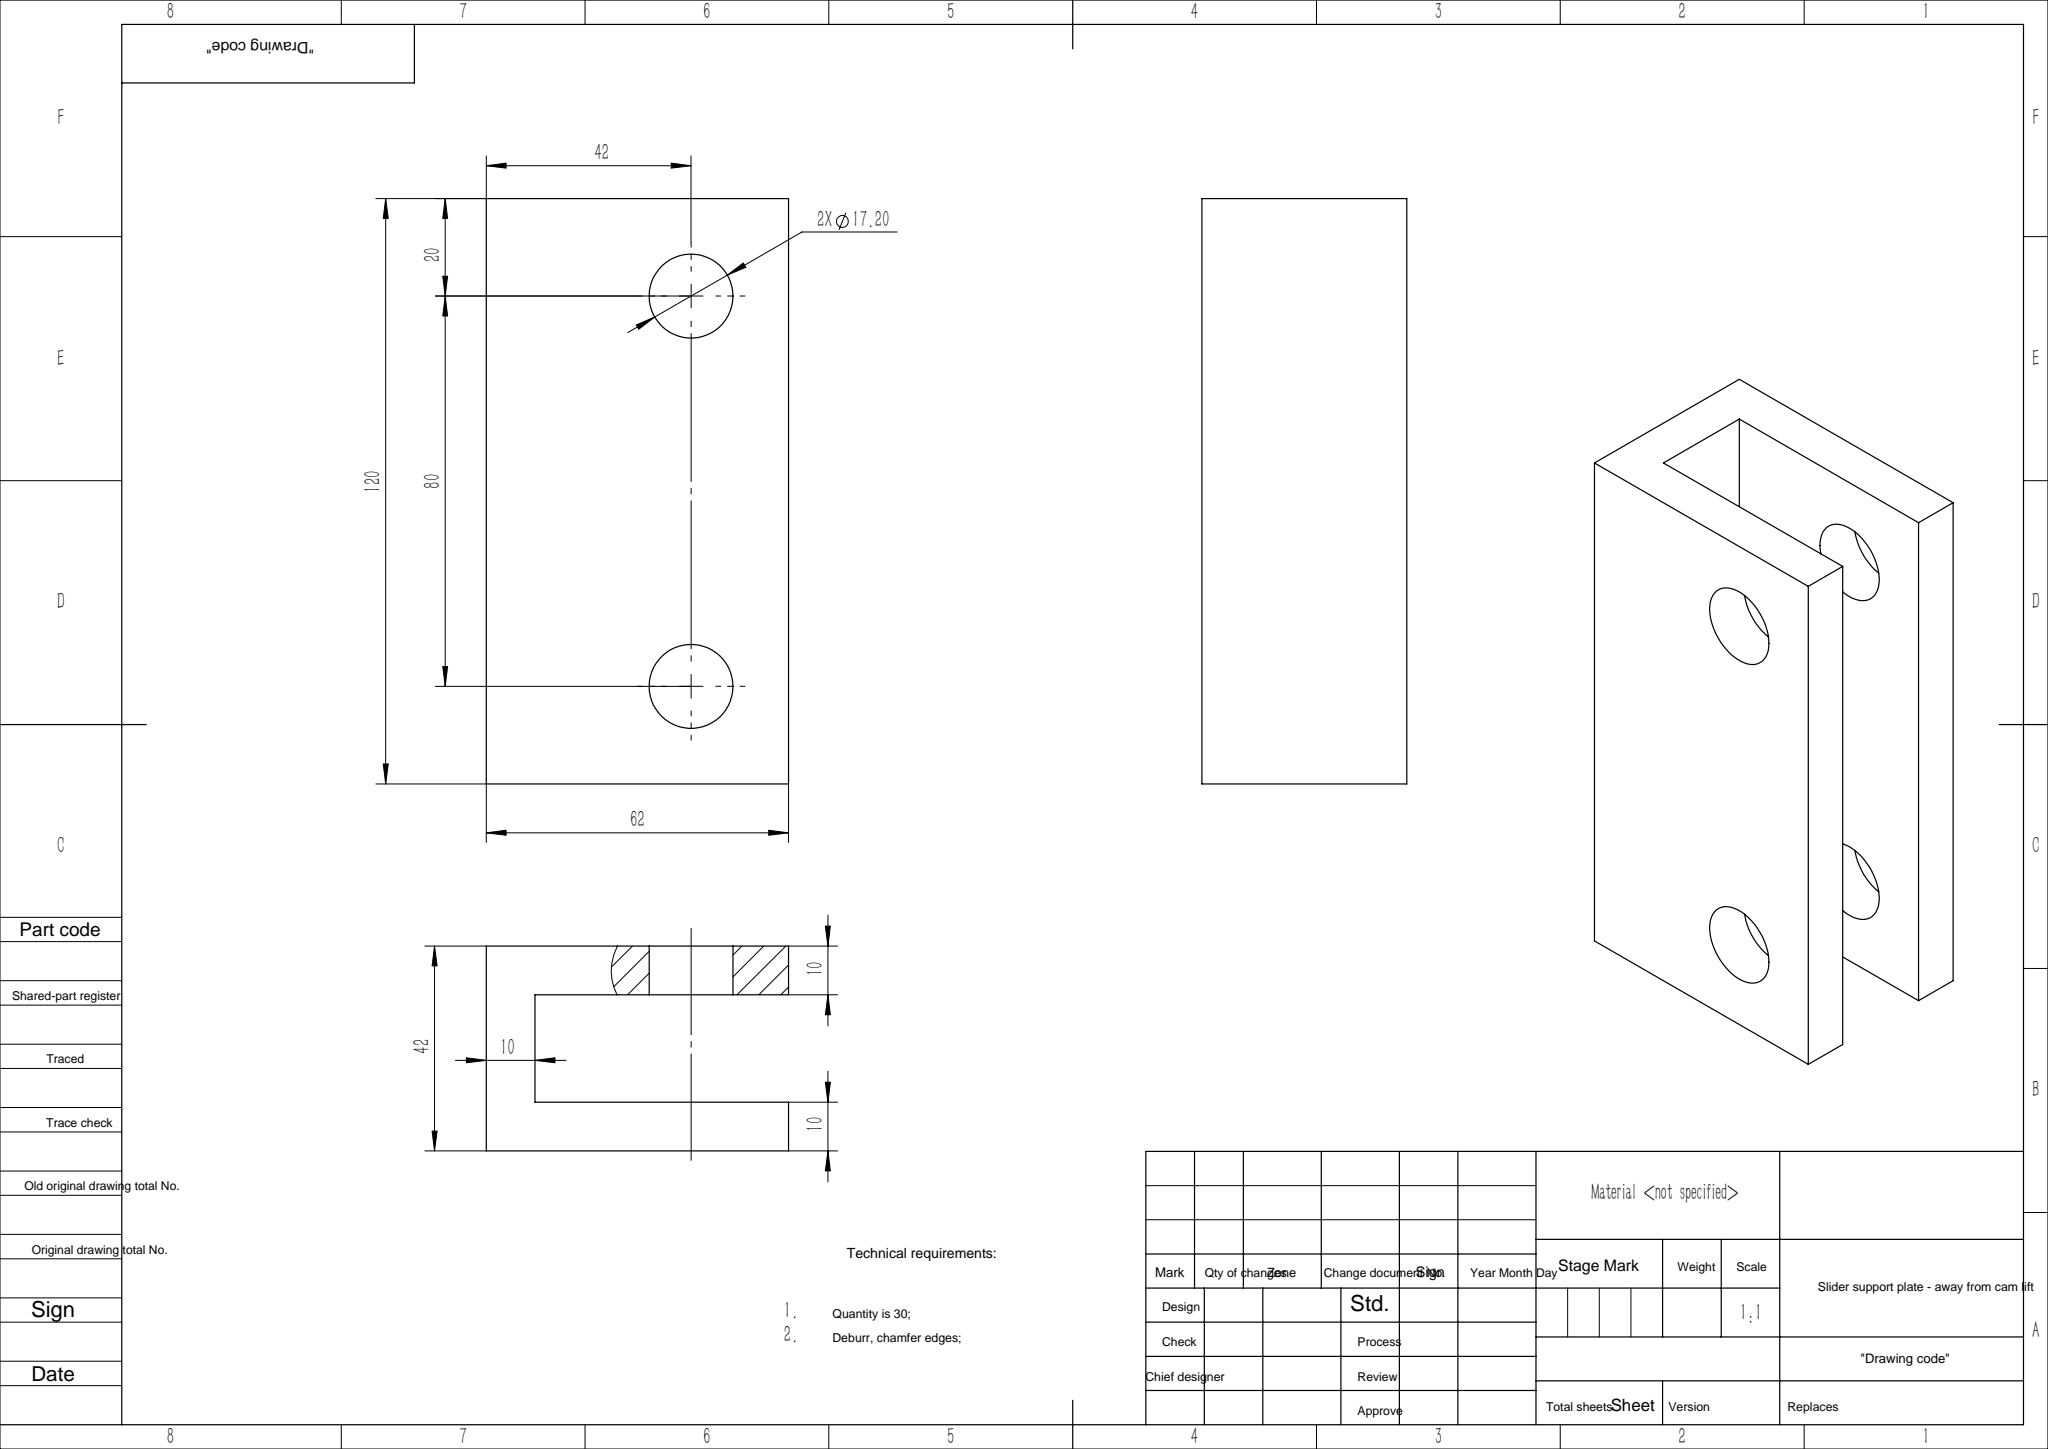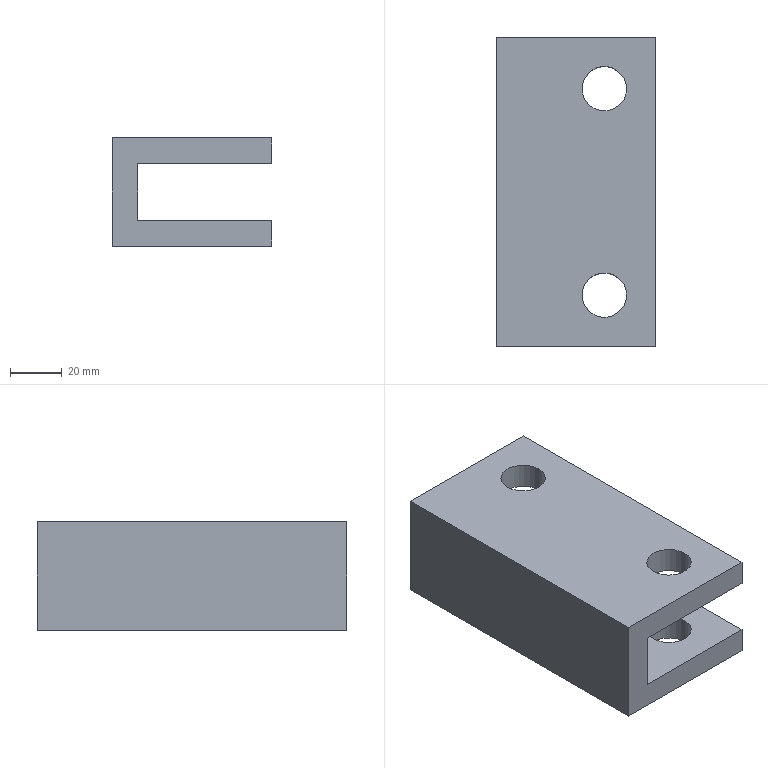Part | SolidWorks | features Extrusion 1, ICE 1 | 1 solid | 18 faces | box 62 x 120 x 42 mm | volume 165906 mm3 | plane 10 | cylinder 8 | commonest cylinder face diameters 17.2 x8
STEP:
#1=CARTESIAN_POINT('',(33.4,20.,11.));
#2=VERTEX_POINT('',#1);
#3=CARTESIAN_POINT('',(50.6,20.,11.));
#4=VERTEX_POINT('',#3);
#5=CARTESIAN_POINT('',(42.,20.,11.));
#6=DIRECTION('',(0.,0.,1.));
#7=DIRECTION('',(1.,0.,0.));
#8=AXIS2_PLACEMENT_3D('',#5,#6,#7);
#9=CIRCLE('',#8,8.6);
#10=EDGE_CURVE('',#2,#4,#9,.T.);
#11=ORIENTED_EDGE('',*,*,#10,.F.);
#12=CARTESIAN_POINT('',(33.4,20.,21.));
#13=VERTEX_POINT('',#12);
#14=CARTESIAN_POINT('',(33.4,20.,-21.));
#15=DIRECTION('',(0.,0.,1.));
#16=VECTOR('',#15,1000.);
#17=LINE('',#14,#16);
#18=EDGE_CURVE('',#2,#13,#17,.T.);
#19=ORIENTED_EDGE('',*,*,#18,.T.);
#20=CARTESIAN_POINT('',(50.6,20.,21.));
#21=VERTEX_POINT('',#20);
#22=CARTESIAN_POINT('',(42.,20.,21.));
#23=DIRECTION('',(0.,0.,1.));
#24=DIRECTION('',(1.,0.,0.));
#25=AXIS2_PLACEMENT_3D('',#22,#23,#24);
#26=CIRCLE('',#25,8.6);
#27=EDGE_CURVE('',#13,#21,#26,.T.);
#28=ORIENTED_EDGE('',*,*,#27,.T.);
#29=CARTESIAN_POINT('',(50.6,20.,-21.));
#30=DIRECTION('',(0.,0.,1.));
#31=VECTOR('',#30,1000.);
#32=LINE('',#29,#31);
#33=EDGE_CURVE('',#4,#21,#32,.T.);
#34=ORIENTED_EDGE('',*,*,#33,.F.);
#35=EDGE_LOOP('',(#11,#19,#28,#34));
#36=FACE_OUTER_BOUND('',#35,.T.);
#37=CARTESIAN_POINT('',(42.,20.,-21.));
#38=DIRECTION('',(0.,0.,1.));
#39=DIRECTION('',(1.,0.,0.));
#40=AXIS2_PLACEMENT_3D('',#37,#38,#39);
#41=CYLINDRICAL_SURFACE('',#40,8.6);
#42=ADVANCED_FACE('',(#36),#41,.F.);
#43=CARTESIAN_POINT('',(33.4,20.,-21.));
#44=VERTEX_POINT('',#43);
#45=CARTESIAN_POINT('',(50.6,20.,-21.));
#46=VERTEX_POINT('',#45);
#47=CARTESIAN_POINT('',(42.,20.,-21.));
#48=DIRECTION('',(0.,0.,1.));
#49=DIRECTION('',(1.,0.,0.));
#50=AXIS2_PLACEMENT_3D('',#47,#48,#49);
#51=CIRCLE('',#50,8.6);
#52=EDGE_CURVE('',#44,#46,#51,.T.);
#53=ORIENTED_EDGE('',*,*,#52,.F.);
#54=CARTESIAN_POINT('',(33.4,20.,-11.));
#55=VERTEX_POINT('',#54);
#56=CARTESIAN_POINT('',(33.4,20.,-21.));
#57=DIRECTION('',(0.,0.,1.));
#58=VECTOR('',#57,1000.);
#59=LINE('',#56,#58);
#60=EDGE_CURVE('',#44,#55,#59,.T.);
#61=ORIENTED_EDGE('',*,*,#60,.T.);
#62=CARTESIAN_POINT('',(50.6,20.,-11.));
#63=VERTEX_POINT('',#62);
#64=CARTESIAN_POINT('',(42.,20.,-11.));
#65=DIRECTION('',(0.,0.,-1.));
#66=DIRECTION('',(-1.,0.,0.));
#67=AXIS2_PLACEMENT_3D('',#64,#65,#66);
#68=CIRCLE('',#67,8.6);
#69=EDGE_CURVE('',#63,#55,#68,.T.);
#70=ORIENTED_EDGE('',*,*,#69,.F.);
#71=CARTESIAN_POINT('',(50.6,20.,-21.));
#72=DIRECTION('',(0.,0.,1.));
#73=VECTOR('',#72,1000.);
#74=LINE('',#71,#73);
#75=EDGE_CURVE('',#46,#63,#74,.T.);
#76=ORIENTED_EDGE('',*,*,#75,.F.);
#77=EDGE_LOOP('',(#53,#61,#70,#76));
#78=FACE_OUTER_BOUND('',#77,.T.);
#79=CARTESIAN_POINT('',(42.,20.,-21.));
#80=DIRECTION('',(0.,0.,1.));
#81=DIRECTION('',(1.,0.,0.));
#82=AXIS2_PLACEMENT_3D('',#79,#80,#81);
#83=CYLINDRICAL_SURFACE('',#82,8.6);
#84=ADVANCED_FACE('',(#78),#83,.F.);
#85=CARTESIAN_POINT('',(33.4,100.,11.));
#86=VERTEX_POINT('',#85);
#87=CARTESIAN_POINT('',(50.6,100.,11.));
#88=VERTEX_POINT('',#87);
#89=CARTESIAN_POINT('',(42.,100.,11.));
#90=DIRECTION('',(0.,0.,1.));
#91=DIRECTION('',(1.,0.,0.));
#92=AXIS2_PLACEMENT_3D('',#89,#90,#91);
#93=CIRCLE('',#92,8.6);
#94=EDGE_CURVE('',#86,#88,#93,.T.);
#95=ORIENTED_EDGE('',*,*,#94,.F.);
#96=CARTESIAN_POINT('',(33.4,100.,21.));
#97=VERTEX_POINT('',#96);
#98=CARTESIAN_POINT('',(33.4,100.,-21.));
#99=DIRECTION('',(0.,0.,1.));
#100=VECTOR('',#99,1000.);
#101=LINE('',#98,#100);
#102=EDGE_CURVE('',#86,#97,#101,.T.);
#103=ORIENTED_EDGE('',*,*,#102,.T.);
#104=CARTESIAN_POINT('',(50.6,100.,21.));
#105=VERTEX_POINT('',#104);
#106=CARTESIAN_POINT('',(42.,100.,21.));
#107=DIRECTION('',(0.,0.,1.));
#108=DIRECTION('',(1.,0.,0.));
#109=AXIS2_PLACEMENT_3D('',#106,#107,#108);
#110=CIRCLE('',#109,8.6);
#111=EDGE_CURVE('',#97,#105,#110,.T.);
#112=ORIENTED_EDGE('',*,*,#111,.T.);
#113=CARTESIAN_POINT('',(50.6,100.,-21.));
#114=DIRECTION('',(0.,0.,1.));
#115=VECTOR('',#114,1000.);
#116=LINE('',#113,#115);
#117=EDGE_CURVE('',#88,#105,#116,.T.);
#118=ORIENTED_EDGE('',*,*,#117,.F.);
#119=EDGE_LOOP('',(#95,#103,#112,#118));
#120=FACE_OUTER_BOUND('',#119,.T.);
#121=CARTESIAN_POINT('',(42.,100.,-21.));
#122=DIRECTION('',(0.,0.,1.));
#123=DIRECTION('',(1.,0.,0.));
#124=AXIS2_PLACEMENT_3D('',#121,#122,#123);
#125=CYLINDRICAL_SURFACE('',#124,8.6);
#126=ADVANCED_FACE('',(#120),#125,.F.);
#127=CARTESIAN_POINT('',(33.4,100.,-21.));
#128=VERTEX_POINT('',#127);
#129=CARTESIAN_POINT('',(50.6,100.,-21.));
#130=VERTEX_POINT('',#129);
#131=CARTESIAN_POINT('',(42.,100.,-21.));
#132=DIRECTION('',(0.,0.,1.));
#133=DIRECTION('',(1.,0.,0.));
#134=AXIS2_PLACEMENT_3D('',#131,#132,#133);
#135=CIRCLE('',#134,8.6);
#136=EDGE_CURVE('',#128,#130,#135,.T.);
#137=ORIENTED_EDGE('',*,*,#136,.F.);
#138=CARTESIAN_POINT('',(33.4,100.,-11.));
#139=VERTEX_POINT('',#138);
#140=CARTESIAN_POINT('',(33.4,100.,-21.));
#141=DIRECTION('',(0.,0.,1.));
#142=VECTOR('',#141,1000.);
#143=LINE('',#140,#142);
#144=EDGE_CURVE('',#128,#139,#143,.T.);
#145=ORIENTED_EDGE('',*,*,#144,.T.);
#146=CARTESIAN_POINT('',(50.6,100.,-11.));
#147=VERTEX_POINT('',#146);
#148=CARTESIAN_POINT('',(42.,100.,-11.));
#149=DIRECTION('',(0.,0.,-1.));
#150=DIRECTION('',(-1.,0.,0.));
#151=AXIS2_PLACEMENT_3D('',#148,#149,#150);
#152=CIRCLE('',#151,8.6);
#153=EDGE_CURVE('',#147,#139,#152,.T.);
#154=ORIENTED_EDGE('',*,*,#153,.F.);
#155=CARTESIAN_POINT('',(50.6,100.,-21.));
#156=DIRECTION('',(0.,0.,1.));
#157=VECTOR('',#156,1000.);
#158=LINE('',#155,#157);
#159=EDGE_CURVE('',#130,#147,#158,.T.);
#160=ORIENTED_EDGE('',*,*,#159,.F.);
#161=EDGE_LOOP('',(#137,#145,#154,#160));
#162=FACE_OUTER_BOUND('',#161,.T.);
#163=CARTESIAN_POINT('',(42.,100.,-21.));
#164=DIRECTION('',(0.,0.,1.));
#165=DIRECTION('',(1.,0.,0.));
#166=AXIS2_PLACEMENT_3D('',#163,#164,#165);
#167=CYLINDRICAL_SURFACE('',#166,8.6);
#168=ADVANCED_FACE('',(#162),#167,.F.);
#169=CARTESIAN_POINT('',(0.,0.,-21.));
#170=VERTEX_POINT('',#169);
#171=CARTESIAN_POINT('',(0.,0.,21.));
#172=VERTEX_POINT('',#171);
#173=CARTESIAN_POINT('',(0.,0.,-21.));
#174=DIRECTION('',(0.,0.,1.));
#175=VECTOR('',#174,1000.);
#176=LINE('',#173,#175);
#177=EDGE_CURVE('',#170,#172,#176,.T.);
#178=ORIENTED_EDGE('',*,*,#177,.T.);
#179=CARTESIAN_POINT('',(0.,120.,21.));
#180=VERTEX_POINT('',#179);
#181=CARTESIAN_POINT('',(0.,120.,21.));
#182=DIRECTION('',(0.,-1.,0.));
#183=VECTOR('',#182,1000.);
#184=LINE('',#181,#183);
#185=EDGE_CURVE('',#180,#172,#184,.T.);
#186=ORIENTED_EDGE('',*,*,#185,.F.);
#187=CARTESIAN_POINT('',(0.,120.,-21.));
#188=VERTEX_POINT('',#187);
#189=CARTESIAN_POINT('',(0.,120.,-21.));
#190=DIRECTION('',(0.,0.,1.));
#191=VECTOR('',#190,1000.);
#192=LINE('',#189,#191);
#193=EDGE_CURVE('',#188,#180,#192,.T.);
#194=ORIENTED_EDGE('',*,*,#193,.F.);
#195=CARTESIAN_POINT('',(0.,120.,-21.));
#196=DIRECTION('',(0.,-1.,0.));
#197=VECTOR('',#196,1000.);
#198=LINE('',#195,#197);
#199=EDGE_CURVE('',#188,#170,#198,.T.);
#200=ORIENTED_EDGE('',*,*,#199,.T.);
#201=EDGE_LOOP('',(#178,#186,#194,#200));
#202=FACE_OUTER_BOUND('',#201,.T.);
#203=CARTESIAN_POINT('',(0.,120.,-21.));
#204=DIRECTION('',(1.,0.,0.));
#205=DIRECTION('',(0.,0.,-1.));
#206=AXIS2_PLACEMENT_3D('',#203,#204,#205);
#207=PLANE('',#206);
#208=ADVANCED_FACE('',(#202),#207,.F.);
#209=CARTESIAN_POINT('',(42.,20.,21.));
#210=DIRECTION('',(0.,0.,1.));
#211=DIRECTION('',(1.,0.,0.));
#212=AXIS2_PLACEMENT_3D('',#209,#210,#211);
#213=CIRCLE('',#212,8.6);
#214=EDGE_CURVE('',#21,#13,#213,.T.);
#215=ORIENTED_EDGE('',*,*,#214,.F.);
#216=ORIENTED_EDGE('',*,*,#27,.F.);
#217=EDGE_LOOP('',(#215,#216));
#218=FACE_BOUND('',#217,.T.);
#219=CARTESIAN_POINT('',(42.,100.,21.));
#220=DIRECTION('',(0.,0.,1.));
#221=DIRECTION('',(1.,0.,0.));
#222=AXIS2_PLACEMENT_3D('',#219,#220,#221);
#223=CIRCLE('',#222,8.6);
#224=EDGE_CURVE('',#105,#97,#223,.T.);
#225=ORIENTED_EDGE('',*,*,#224,.F.);
#226=ORIENTED_EDGE('',*,*,#111,.F.);
#227=EDGE_LOOP('',(#225,#226));
#228=FACE_BOUND('',#227,.T.);
#229=CARTESIAN_POINT('',(62.,0.,21.));
#230=VERTEX_POINT('',#229);
#231=CARTESIAN_POINT('',(0.,0.,21.));
#232=DIRECTION('',(1.,0.,0.));
#233=VECTOR('',#232,1000.);
#234=LINE('',#231,#233);
#235=EDGE_CURVE('',#172,#230,#234,.T.);
#236=ORIENTED_EDGE('',*,*,#235,.T.);
#237=CARTESIAN_POINT('',(62.,120.,21.));
#238=VERTEX_POINT('',#237);
#239=CARTESIAN_POINT('',(62.,120.,21.));
#240=DIRECTION('',(0.,-1.,0.));
#241=VECTOR('',#240,1000.);
#242=LINE('',#239,#241);
#243=EDGE_CURVE('',#238,#230,#242,.T.);
#244=ORIENTED_EDGE('',*,*,#243,.F.);
#245=CARTESIAN_POINT('',(0.,120.,21.));
#246=DIRECTION('',(1.,0.,0.));
#247=VECTOR('',#246,1000.);
#248=LINE('',#245,#247);
#249=EDGE_CURVE('',#180,#238,#248,.T.);
#250=ORIENTED_EDGE('',*,*,#249,.F.);
#251=ORIENTED_EDGE('',*,*,#185,.T.);
#252=EDGE_LOOP('',(#236,#244,#250,#251));
#253=FACE_OUTER_BOUND('',#252,.T.);
#254=CARTESIAN_POINT('',(0.,120.,21.));
#255=DIRECTION('',(0.,0.,-1.));
#256=DIRECTION('',(-1.,0.,0.));
#257=AXIS2_PLACEMENT_3D('',#254,#255,#256);
#258=PLANE('',#257);
#259=ADVANCED_FACE('',(#218,#228,#253),#258,.F.);
#260=CARTESIAN_POINT('',(62.,0.,11.));
#261=VERTEX_POINT('',#260);
#262=CARTESIAN_POINT('',(62.,0.,11.));
#263=DIRECTION('',(0.,0.,-1.));
#264=VECTOR('',#263,1000.);
#265=LINE('',#262,#264);
#266=EDGE_CURVE('',#230,#261,#265,.T.);
#267=ORIENTED_EDGE('',*,*,#266,.T.);
#268=CARTESIAN_POINT('',(62.,120.,11.));
#269=VERTEX_POINT('',#268);
#270=CARTESIAN_POINT('',(62.,120.,11.));
#271=DIRECTION('',(0.,-1.,0.));
#272=VECTOR('',#271,1000.);
#273=LINE('',#270,#272);
#274=EDGE_CURVE('',#269,#261,#273,.T.);
#275=ORIENTED_EDGE('',*,*,#274,.F.);
#276=CARTESIAN_POINT('',(62.,120.,11.));
#277=DIRECTION('',(0.,0.,-1.));
#278=VECTOR('',#277,1000.);
#279=LINE('',#276,#278);
#280=EDGE_CURVE('',#238,#269,#279,.T.);
#281=ORIENTED_EDGE('',*,*,#280,.F.);
#282=ORIENTED_EDGE('',*,*,#243,.T.);
#283=EDGE_LOOP('',(#267,#275,#281,#282));
#284=FACE_OUTER_BOUND('',#283,.T.);
#285=CARTESIAN_POINT('',(62.,120.,11.));
#286=DIRECTION('',(-1.,0.,0.));
#287=DIRECTION('',(0.,0.,1.));
#288=AXIS2_PLACEMENT_3D('',#285,#286,#287);
#289=PLANE('',#288);
#290=ADVANCED_FACE('',(#284),#289,.F.);
#291=CARTESIAN_POINT('',(42.,20.,11.));
#292=DIRECTION('',(0.,0.,1.));
#293=DIRECTION('',(1.,0.,0.));
#294=AXIS2_PLACEMENT_3D('',#291,#292,#293);
#295=CIRCLE('',#294,8.6);
#296=EDGE_CURVE('',#4,#2,#295,.T.);
#297=ORIENTED_EDGE('',*,*,#296,.T.);
#298=ORIENTED_EDGE('',*,*,#10,.T.);
#299=EDGE_LOOP('',(#297,#298));
#300=FACE_BOUND('',#299,.T.);
#301=CARTESIAN_POINT('',(42.,100.,11.));
#302=DIRECTION('',(0.,0.,1.));
#303=DIRECTION('',(1.,0.,0.));
#304=AXIS2_PLACEMENT_3D('',#301,#302,#303);
#305=CIRCLE('',#304,8.6);
#306=EDGE_CURVE('',#88,#86,#305,.T.);
#307=ORIENTED_EDGE('',*,*,#306,.T.);
#308=ORIENTED_EDGE('',*,*,#94,.T.);
#309=EDGE_LOOP('',(#307,#308));
#310=FACE_BOUND('',#309,.T.);
#311=CARTESIAN_POINT('',(10.,0.,11.));
#312=VERTEX_POINT('',#311);
#313=CARTESIAN_POINT('',(10.,0.,11.));
#314=DIRECTION('',(-1.,0.,0.));
#315=VECTOR('',#314,1000.);
#316=LINE('',#313,#315);
#317=EDGE_CURVE('',#261,#312,#316,.T.);
#318=ORIENTED_EDGE('',*,*,#317,.T.);
#319=CARTESIAN_POINT('',(10.,120.,11.));
#320=VERTEX_POINT('',#319);
#321=CARTESIAN_POINT('',(10.,120.,11.));
#322=DIRECTION('',(0.,-1.,0.));
#323=VECTOR('',#322,1000.);
#324=LINE('',#321,#323);
#325=EDGE_CURVE('',#320,#312,#324,.T.);
#326=ORIENTED_EDGE('',*,*,#325,.F.);
#327=CARTESIAN_POINT('',(10.,120.,11.));
#328=DIRECTION('',(-1.,0.,0.));
#329=VECTOR('',#328,1000.);
#330=LINE('',#327,#329);
#331=EDGE_CURVE('',#269,#320,#330,.T.);
#332=ORIENTED_EDGE('',*,*,#331,.F.);
#333=ORIENTED_EDGE('',*,*,#274,.T.);
#334=EDGE_LOOP('',(#318,#326,#332,#333));
#335=FACE_OUTER_BOUND('',#334,.T.);
#336=CARTESIAN_POINT('',(10.,120.,11.));
#337=DIRECTION('',(0.,0.,1.));
#338=DIRECTION('',(1.,0.,0.));
#339=AXIS2_PLACEMENT_3D('',#336,#337,#338);
#340=PLANE('',#339);
#341=ADVANCED_FACE('',(#300,#310,#335),#340,.F.);
#342=CARTESIAN_POINT('',(10.,0.,-11.));
#343=VERTEX_POINT('',#342);
#344=CARTESIAN_POINT('',(10.,0.,-11.));
#345=DIRECTION('',(0.,0.,-1.));
#346=VECTOR('',#345,1000.);
#347=LINE('',#344,#346);
#348=EDGE_CURVE('',#312,#343,#347,.T.);
#349=ORIENTED_EDGE('',*,*,#348,.T.);
#350=CARTESIAN_POINT('',(10.,120.,-11.));
#351=VERTEX_POINT('',#350);
#352=CARTESIAN_POINT('',(10.,120.,-11.));
#353=DIRECTION('',(0.,-1.,0.));
#354=VECTOR('',#353,1000.);
#355=LINE('',#352,#354);
#356=EDGE_CURVE('',#351,#343,#355,.T.);
#357=ORIENTED_EDGE('',*,*,#356,.F.);
#358=CARTESIAN_POINT('',(10.,120.,-11.));
#359=DIRECTION('',(0.,0.,-1.));
#360=VECTOR('',#359,1000.);
#361=LINE('',#358,#360);
#362=EDGE_CURVE('',#320,#351,#361,.T.);
#363=ORIENTED_EDGE('',*,*,#362,.F.);
#364=ORIENTED_EDGE('',*,*,#325,.T.);
#365=EDGE_LOOP('',(#349,#357,#363,#364));
#366=FACE_OUTER_BOUND('',#365,.T.);
#367=CARTESIAN_POINT('',(10.,120.,-11.));
#368=DIRECTION('',(-1.,0.,0.));
#369=DIRECTION('',(0.,0.,1.));
#370=AXIS2_PLACEMENT_3D('',#367,#368,#369);
#371=PLANE('',#370);
#372=ADVANCED_FACE('',(#366),#371,.F.);
#373=ORIENTED_EDGE('',*,*,#69,.T.);
#374=CARTESIAN_POINT('',(42.,20.,-11.));
#375=DIRECTION('',(0.,0.,-1.));
#376=DIRECTION('',(-1.,0.,0.));
#377=AXIS2_PLACEMENT_3D('',#374,#375,#376);
#378=CIRCLE('',#377,8.6);
#379=EDGE_CURVE('',#55,#63,#378,.T.);
#380=ORIENTED_EDGE('',*,*,#379,.T.);
#381=EDGE_LOOP('',(#373,#380));
#382=FACE_BOUND('',#381,.T.);
#383=ORIENTED_EDGE('',*,*,#153,.T.);
#384=CARTESIAN_POINT('',(42.,100.,-11.));
#385=DIRECTION('',(0.,0.,-1.));
#386=DIRECTION('',(-1.,0.,0.));
#387=AXIS2_PLACEMENT_3D('',#384,#385,#386);
#388=CIRCLE('',#387,8.6);
#389=EDGE_CURVE('',#139,#147,#388,.T.);
#390=ORIENTED_EDGE('',*,*,#389,.T.);
#391=EDGE_LOOP('',(#383,#390));
#392=FACE_BOUND('',#391,.T.);
#393=CARTESIAN_POINT('',(62.,0.,-11.));
#394=VERTEX_POINT('',#393);
#395=CARTESIAN_POINT('',(62.,0.,-11.));
#396=DIRECTION('',(1.,0.,0.));
#397=VECTOR('',#396,1000.);
#398=LINE('',#395,#397);
#399=EDGE_CURVE('',#343,#394,#398,.T.);
#400=ORIENTED_EDGE('',*,*,#399,.T.);
#401=CARTESIAN_POINT('',(62.,120.,-11.));
#402=VERTEX_POINT('',#401);
#403=CARTESIAN_POINT('',(62.,120.,-11.));
#404=DIRECTION('',(0.,-1.,0.));
#405=VECTOR('',#404,1000.);
#406=LINE('',#403,#405);
#407=EDGE_CURVE('',#402,#394,#406,.T.);
#408=ORIENTED_EDGE('',*,*,#407,.F.);
#409=CARTESIAN_POINT('',(62.,120.,-11.));
#410=DIRECTION('',(1.,0.,0.));
#411=VECTOR('',#410,1000.);
#412=LINE('',#409,#411);
#413=EDGE_CURVE('',#351,#402,#412,.T.);
#414=ORIENTED_EDGE('',*,*,#413,.F.);
#415=ORIENTED_EDGE('',*,*,#356,.T.);
#416=EDGE_LOOP('',(#400,#408,#414,#415));
#417=FACE_OUTER_BOUND('',#416,.T.);
#418=CARTESIAN_POINT('',(62.,120.,-11.));
#419=DIRECTION('',(0.,0.,-1.));
#420=DIRECTION('',(-1.,0.,0.));
#421=AXIS2_PLACEMENT_3D('',#418,#419,#420);
#422=PLANE('',#421);
#423=ADVANCED_FACE('',(#382,#392,#417),#422,.F.);
#424=CARTESIAN_POINT('',(62.,0.,-21.));
#425=VERTEX_POINT('',#424);
#426=CARTESIAN_POINT('',(62.,0.,-21.));
#427=DIRECTION('',(0.,0.,-1.));
#428=VECTOR('',#427,1000.);
#429=LINE('',#426,#428);
#430=EDGE_CURVE('',#394,#425,#429,.T.);
#431=ORIENTED_EDGE('',*,*,#430,.T.);
#432=CARTESIAN_POINT('',(62.,120.,-21.));
#433=VERTEX_POINT('',#432);
#434=CARTESIAN_POINT('',(62.,120.,-21.));
#435=DIRECTION('',(0.,-1.,0.));
#436=VECTOR('',#435,1000.);
#437=LINE('',#434,#436);
#438=EDGE_CURVE('',#433,#425,#437,.T.);
#439=ORIENTED_EDGE('',*,*,#438,.F.);
#440=CARTESIAN_POINT('',(62.,120.,-21.));
#441=DIRECTION('',(0.,0.,-1.));
#442=VECTOR('',#441,1000.);
#443=LINE('',#440,#442);
#444=EDGE_CURVE('',#402,#433,#443,.T.);
#445=ORIENTED_EDGE('',*,*,#444,.F.);
#446=ORIENTED_EDGE('',*,*,#407,.T.);
#447=EDGE_LOOP('',(#431,#439,#445,#446));
#448=FACE_OUTER_BOUND('',#447,.T.);
#449=CARTESIAN_POINT('',(62.,120.,-21.));
#450=DIRECTION('',(-1.,0.,0.));
#451=DIRECTION('',(0.,0.,1.));
#452=AXIS2_PLACEMENT_3D('',#449,#450,#451);
#453=PLANE('',#452);
#454=ADVANCED_FACE('',(#448),#453,.F.);
#455=CARTESIAN_POINT('',(42.,20.,-21.));
#456=DIRECTION('',(0.,0.,1.));
#457=DIRECTION('',(1.,0.,0.));
#458=AXIS2_PLACEMENT_3D('',#455,#456,#457);
#459=CIRCLE('',#458,8.6);
#460=EDGE_CURVE('',#46,#44,#459,.T.);
#461=ORIENTED_EDGE('',*,*,#460,.T.);
#462=ORIENTED_EDGE('',*,*,#52,.T.);
#463=EDGE_LOOP('',(#461,#462));
#464=FACE_BOUND('',#463,.T.);
#465=CARTESIAN_POINT('',(42.,100.,-21.));
#466=DIRECTION('',(0.,0.,1.));
#467=DIRECTION('',(1.,0.,0.));
#468=AXIS2_PLACEMENT_3D('',#465,#466,#467);
#469=CIRCLE('',#468,8.6);
#470=EDGE_CURVE('',#130,#128,#469,.T.);
#471=ORIENTED_EDGE('',*,*,#470,.T.);
#472=ORIENTED_EDGE('',*,*,#136,.T.);
#473=EDGE_LOOP('',(#471,#472));
#474=FACE_BOUND('',#473,.T.);
#475=CARTESIAN_POINT('',(0.,0.,-21.));
#476=DIRECTION('',(-1.,0.,0.));
#477=VECTOR('',#476,1000.);
#478=LINE('',#475,#477);
#479=EDGE_CURVE('',#425,#170,#478,.T.);
#480=ORIENTED_EDGE('',*,*,#479,.T.);
#481=ORIENTED_EDGE('',*,*,#199,.F.);
#482=CARTESIAN_POINT('',(0.,120.,-21.));
#483=DIRECTION('',(-1.,0.,0.));
#484=VECTOR('',#483,1000.);
#485=LINE('',#482,#484);
#486=EDGE_CURVE('',#433,#188,#485,.T.);
#487=ORIENTED_EDGE('',*,*,#486,.F.);
#488=ORIENTED_EDGE('',*,*,#438,.T.);
#489=EDGE_LOOP('',(#480,#481,#487,#488));
#490=FACE_OUTER_BOUND('',#489,.T.);
#491=CARTESIAN_POINT('',(0.,120.,-21.));
#492=DIRECTION('',(0.,0.,1.));
#493=DIRECTION('',(1.,0.,0.));
#494=AXIS2_PLACEMENT_3D('',#491,#492,#493);
#495=PLANE('',#494);
#496=ADVANCED_FACE('',(#464,#474,#490),#495,.F.);
#497=ORIENTED_EDGE('',*,*,#193,.T.);
#498=ORIENTED_EDGE('',*,*,#249,.T.);
#499=ORIENTED_EDGE('',*,*,#280,.T.);
#500=ORIENTED_EDGE('',*,*,#331,.T.);
#501=ORIENTED_EDGE('',*,*,#362,.T.);
#502=ORIENTED_EDGE('',*,*,#413,.T.);
#503=ORIENTED_EDGE('',*,*,#444,.T.);
#504=ORIENTED_EDGE('',*,*,#486,.T.);
#505=EDGE_LOOP('',(#497,#498,#499,#500,#501,#502,#503,#504));
#506=FACE_OUTER_BOUND('',#505,.T.);
#507=CARTESIAN_POINT('',(0.,120.,0.));
#508=DIRECTION('',(0.,1.,0.));
#509=DIRECTION('',(0.,0.,1.));
#510=AXIS2_PLACEMENT_3D('',#507,#508,#509);
#511=PLANE('',#510);
#512=ADVANCED_FACE('',(#506),#511,.T.);
#513=ORIENTED_EDGE('',*,*,#177,.F.);
#514=ORIENTED_EDGE('',*,*,#479,.F.);
#515=ORIENTED_EDGE('',*,*,#430,.F.);
#516=ORIENTED_EDGE('',*,*,#399,.F.);
#517=ORIENTED_EDGE('',*,*,#348,.F.);
#518=ORIENTED_EDGE('',*,*,#317,.F.);
#519=ORIENTED_EDGE('',*,*,#266,.F.);
#520=ORIENTED_EDGE('',*,*,#235,.F.);
#521=EDGE_LOOP('',(#513,#514,#515,#516,#517,#518,#519,#520));
#522=FACE_OUTER_BOUND('',#521,.T.);
#523=CARTESIAN_POINT('',(0.,0.,0.));
#524=DIRECTION('',(0.,1.,0.));
#525=DIRECTION('',(0.,0.,1.));
#526=AXIS2_PLACEMENT_3D('',#523,#524,#525);
#527=PLANE('',#526);
#528=ADVANCED_FACE('',(#522),#527,.F.);
#529=ORIENTED_EDGE('',*,*,#144,.F.);
#530=ORIENTED_EDGE('',*,*,#470,.F.);
#531=ORIENTED_EDGE('',*,*,#159,.T.);
#532=ORIENTED_EDGE('',*,*,#389,.F.);
#533=EDGE_LOOP('',(#529,#530,#531,#532));
#534=FACE_OUTER_BOUND('',#533,.T.);
#535=CARTESIAN_POINT('',(42.,100.,-21.));
#536=DIRECTION('',(0.,0.,1.));
#537=DIRECTION('',(1.,0.,0.));
#538=AXIS2_PLACEMENT_3D('',#535,#536,#537);
#539=CYLINDRICAL_SURFACE('',#538,8.6);
#540=ADVANCED_FACE('',(#534),#539,.F.);
#541=ORIENTED_EDGE('',*,*,#102,.F.);
#542=ORIENTED_EDGE('',*,*,#306,.F.);
#543=ORIENTED_EDGE('',*,*,#117,.T.);
#544=ORIENTED_EDGE('',*,*,#224,.T.);
#545=EDGE_LOOP('',(#541,#542,#543,#544));
#546=FACE_OUTER_BOUND('',#545,.T.);
#547=CARTESIAN_POINT('',(42.,100.,-21.));
#548=DIRECTION('',(0.,0.,1.));
#549=DIRECTION('',(1.,0.,0.));
#550=AXIS2_PLACEMENT_3D('',#547,#548,#549);
#551=CYLINDRICAL_SURFACE('',#550,8.6);
#552=ADVANCED_FACE('',(#546),#551,.F.);
#553=ORIENTED_EDGE('',*,*,#60,.F.);
#554=ORIENTED_EDGE('',*,*,#460,.F.);
#555=ORIENTED_EDGE('',*,*,#75,.T.);
#556=ORIENTED_EDGE('',*,*,#379,.F.);
#557=EDGE_LOOP('',(#553,#554,#555,#556));
#558=FACE_OUTER_BOUND('',#557,.T.);
#559=CARTESIAN_POINT('',(42.,20.,-21.));
#560=DIRECTION('',(0.,0.,1.));
#561=DIRECTION('',(1.,0.,0.));
#562=AXIS2_PLACEMENT_3D('',#559,#560,#561);
#563=CYLINDRICAL_SURFACE('',#562,8.6);
#564=ADVANCED_FACE('',(#558),#563,.F.);
#565=ORIENTED_EDGE('',*,*,#18,.F.);
#566=ORIENTED_EDGE('',*,*,#296,.F.);
#567=ORIENTED_EDGE('',*,*,#33,.T.);
#568=ORIENTED_EDGE('',*,*,#214,.T.);
#569=EDGE_LOOP('',(#565,#566,#567,#568));
#570=FACE_OUTER_BOUND('',#569,.T.);
#571=CARTESIAN_POINT('',(42.,20.,-21.));
#572=DIRECTION('',(0.,0.,1.));
#573=DIRECTION('',(1.,0.,0.));
#574=AXIS2_PLACEMENT_3D('',#571,#572,#573);
#575=CYLINDRICAL_SURFACE('',#574,8.6);
#576=ADVANCED_FACE('',(#570),#575,.F.);
#577=CLOSED_SHELL('',(#42,#84,#126,#168,#208,#259,#290,#341,#372,#423,#454,#496,#512,#528,#540,#552,#564,#576));
#578=MANIFOLD_SOLID_BREP('',#577);
#579=CARTESIAN_POINT('',(0.,0.,0.));
#580=DIRECTION('',(0.,0.,1.));
#581=DIRECTION('',(1.,0.,0.));
#582=AXIS2_PLACEMENT_3D('',#579,#580,#581);
#583=(LENGTH_UNIT()NAMED_UNIT(*)SI_UNIT(.MILLI.,.METRE.));
#584=UNCERTAINTY_MEASURE_WITH_UNIT(LENGTH_MEASURE(0.00001),#583,'','');
#585=(NAMED_UNIT(*)PLANE_ANGLE_UNIT()SI_UNIT($,.RADIAN.));
#586=(NAMED_UNIT(*)SI_UNIT($,.STERADIAN.)SOLID_ANGLE_UNIT());
#587=(GEOMETRIC_REPRESENTATION_CONTEXT(3)GLOBAL_UNCERTAINTY_ASSIGNED_CONTEXT((#584))GLOBAL_UNIT_ASSIGNED_CONTEXT((#583,#585,#586))REPRESENTATION_CONTEXT('',''));
#588=ADVANCED_BREP_SHAPE_REPRESENTATION('',(#578,#582),#587);